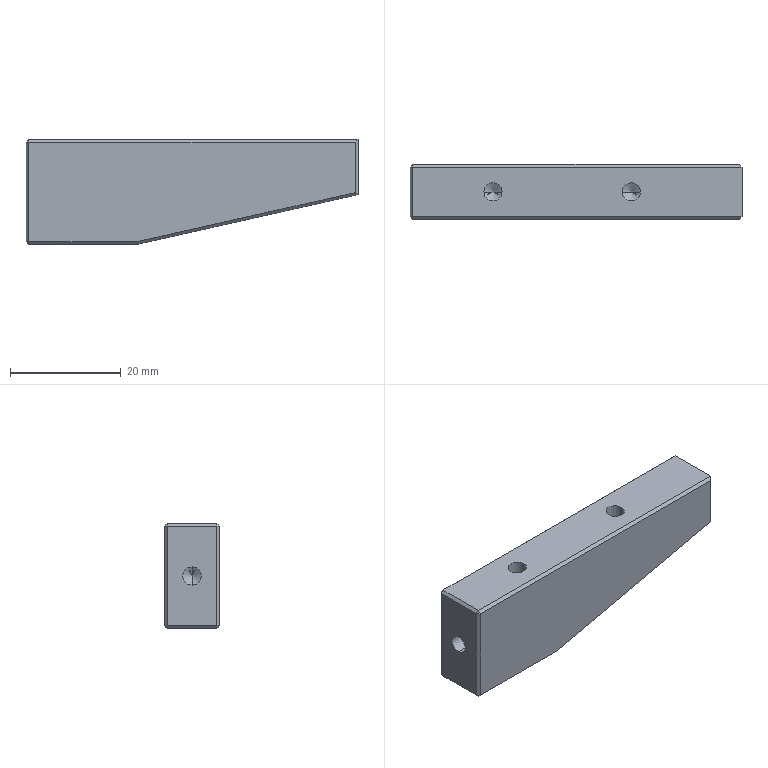Part | STEP file | ND25021-01-JDKM-27-TL | 1 solid | 35 faces | box 60 x 10 x 19 mm | volume 9293 mm3 | plane 23 | cylinder 6 | cone 6 | commonest cylinder face diameters 3.3 x6